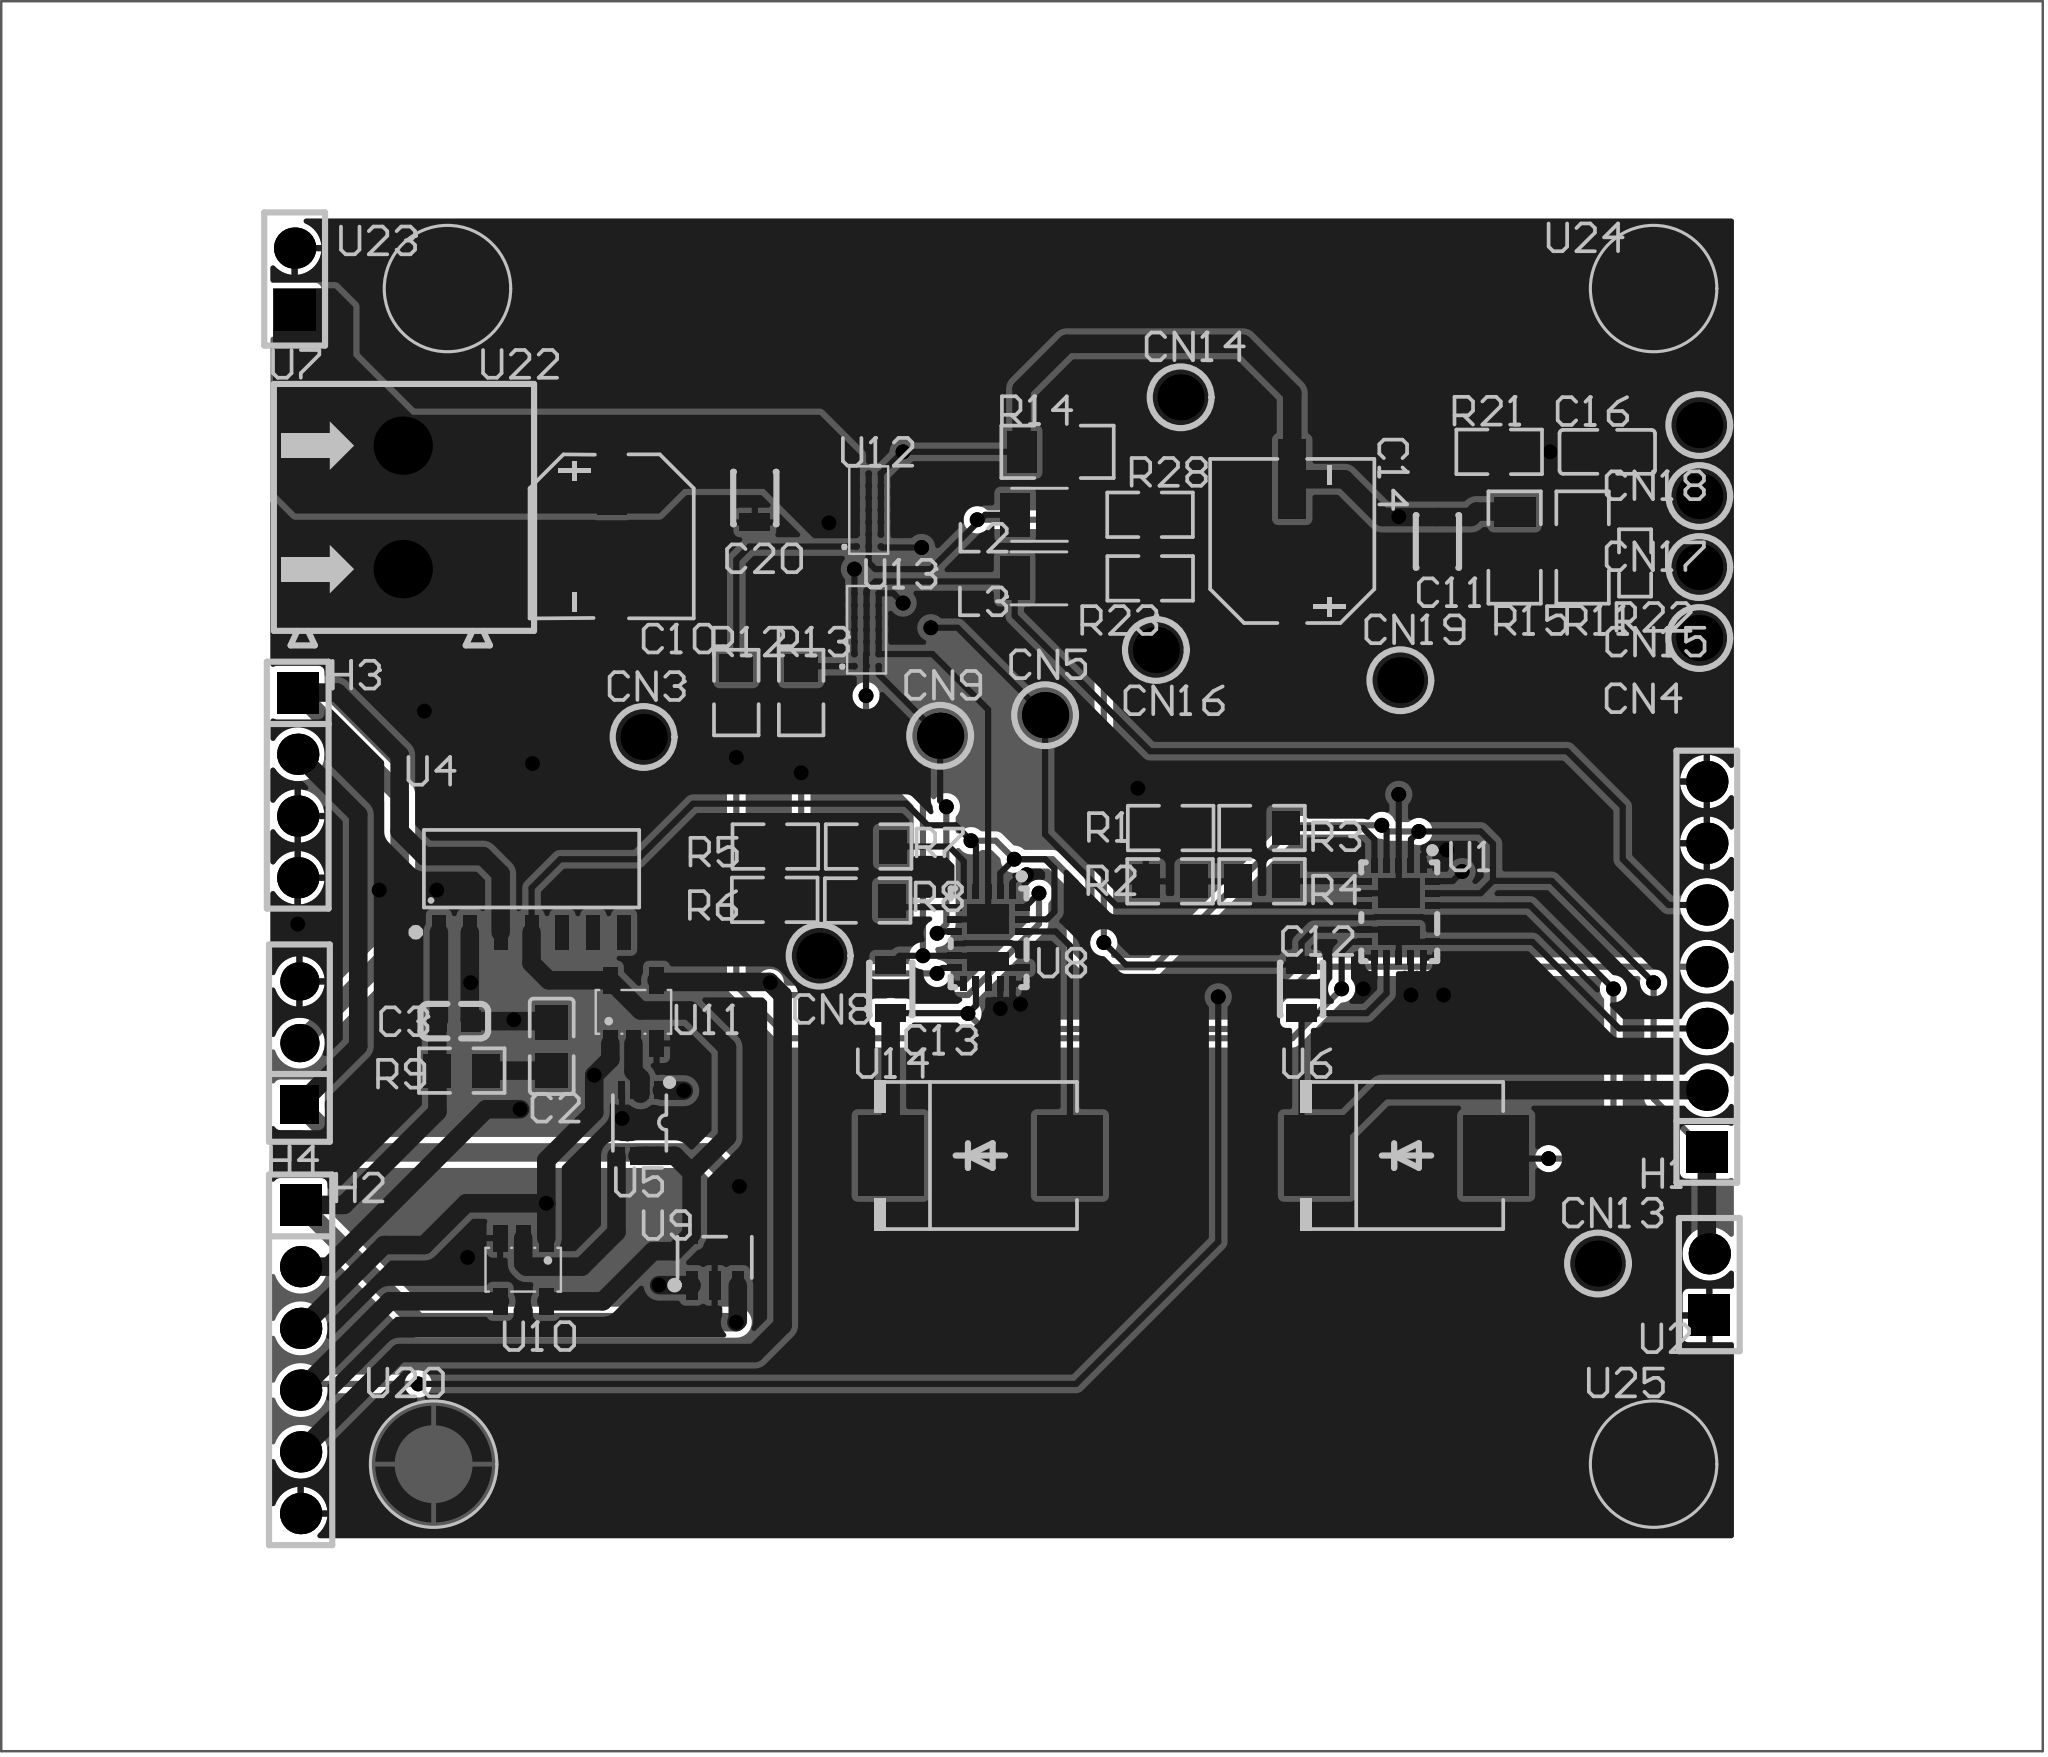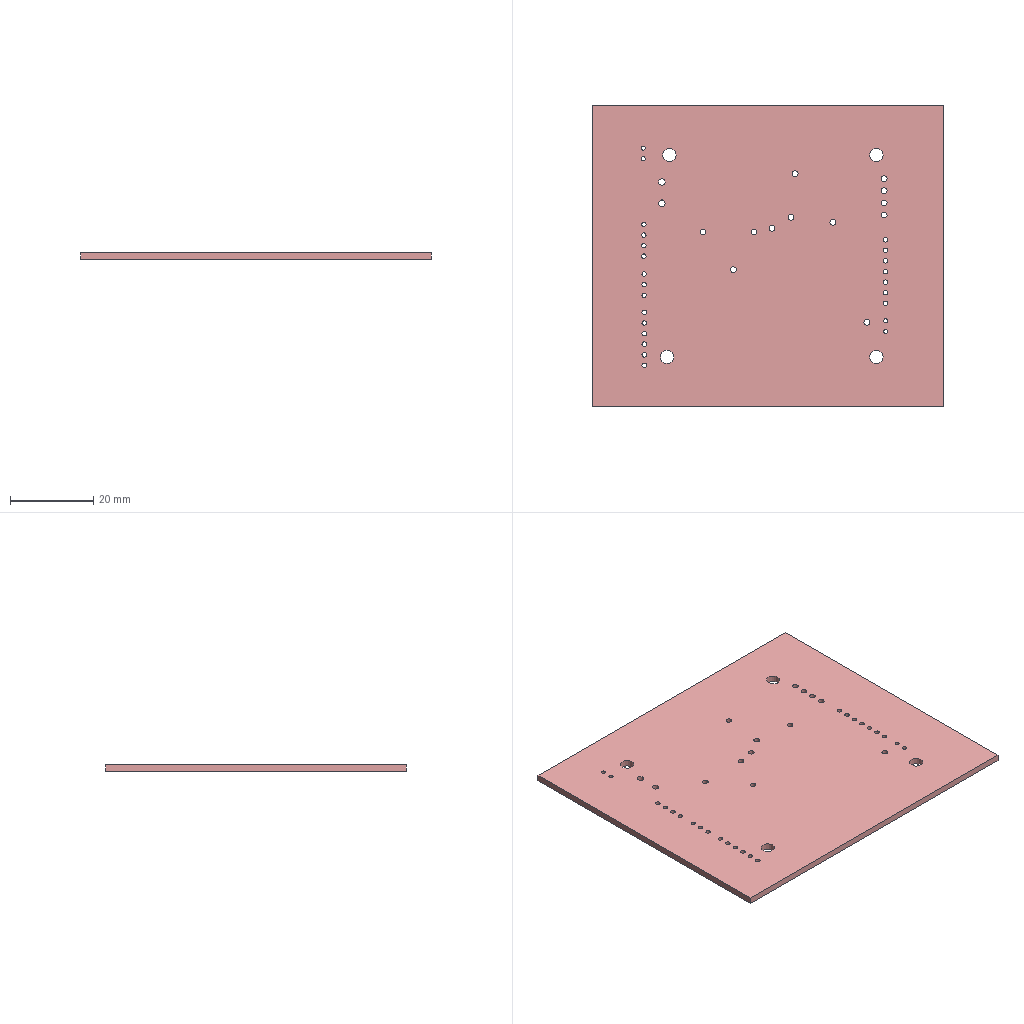Circuit board layout | Altium Designer | box 83.9 x 72 x 1.6 mm
Layer stack:
# Altium Designer layer stack of  (unit mm; dielectric type: 0 none, 1 core, 2 prepreg, 3 surface material)
index,name,kind,layer,copper_thickness_mm,dielectric_type,dielectric_thickness_mm,dielectric_material,dielectric_constant
0,Top Paste Mask Layer,other,,,,,,
1,Top Silkscreen Layer,other,,,,,,
2,Top Solder Mask Layer,dielectric,,,3,0.01,,3.3
3,Top Layer,copper,Top Layer,0.035,,,,
4,Dielectric1,dielectric,,,3,1.51,FR4,4.5
5,Bottom Layer,copper,Bottom Layer,0.035,,,,
6,Bottom Solder Mask Layer,dielectric,,,3,0.01,,3.3
7,Bottom Silkscreen Layer,other,,,,,,
8,Bottom Paste Mask Layer,other,,,,,,
# drill layer pairs: low layer,high layer
drill_pair,Top Layer,Bottom Layer
Part placement:
Designator,Comment,Layer,Footprint,Center-X(mm),Center-Y(mm),Rotation
C2,24pF,TopLayer,C0805,92.485,98.854,90
C3,0.6pF,TopLayer,C0603,88.48,99.891,0
C10,100uF,TopLayer,CAP-SMD_BD6.3-L6.6-W6.6-LS7.3-FD-H7.7,94.95,119.837,270
C11,100nF,TopLayer,CAP-SMD_L2.0-W1.25,128.905,119.634,270
C12,100nF,TopLayer,CAP-SMD_L2.0-W1.25,123.317,101.219,270
C13,100nF,TopLayer,CAP-SMD_L2.0-W1.25,106.426,101.219,270
C14,100uF,TopLayer,CAP-SMD_BD6.3-L6.6-W6.6-RD,122.936,119.634,270
C16,1.2pF,TopLayer,C0805,135.89,123.317,0
C20,100nF,TopLayer,CAP-SMD_L2.0-W1.25,100.838,121.412,90
H1,PZ254V-11-07P,TopLayer,HDR-TH_7P-P2.54-V-M,139.984,102.13,90
H2,PZ254V-11-06P,TopLayer,HDR-TH_6P-P2.54-V-M,82.161,85.979,270
H3,PZ254V-11-04P,TopLayer,HDR-TH_4P-P2.54-V-M,82.042,109.601,270
H4,PM254V-11-03-H85,TopLayer,HDR-TH_3P-P2.54-V-F,82.111,98.987,90
L2,100nH,TopLayer,IND-SMD_L2.3-W1.8,112.541,120.727,0
L3,100nH,TopLayer,IND-SMD_L2.3-W1.8,112.522,118.11,0
R1,120kΩ,TopLayer,R0805,117.936,107.838,0
R2,120kΩ,TopLayer,R0805,117.911,105.644,0
R3,20kΩ,TopLayer,R0805,121.693,107.838,0
R4,20kΩ,TopLayer,R0805,121.693,105.644,0
R5,120kΩ,TopLayer,R0805,101.68,107.076,0
R6,120kΩ,TopLayer,R0805,101.655,104.882,0
R7,20kΩ,TopLayer,R0805,105.516,107.076,0
R8,20kΩ,TopLayer,R0805,105.478,104.854,0
R9,100kΩ,TopLayer,R0805,88.786,97.854,0
R11,900kΩ,TopLayer,R1206,134.874,119.38,270
R12,4.7Ω,TopLayer,R0805,100.076,113.411,90
R13,4.7Ω,TopLayer,R0805,102.743,113.411,90
R14,0Ω,TopLayer,R1206,113.284,123.317,180
R15,600mΩ,TopLayer,R1206,132.08,119.38,270
R21,1.8MΩ,TopLayer,R0805,131.445,123.317,0
R22,69kΩ,TopLayer,R0603,137.033,118.745,270
R23,10mΩ,TopLayer,R0805,117.094,118.11,0
R28,10mΩ,TopLayer,R0805,117.088,120.727,0
U1,LMG1210RVRR,TopLayer,WQFN-19_L4.0-W3.0-P0.50-BL-EP_LMG1210RVRR,127.316,104.403,270
U2,ZX-PM2.54-1-2PY,TopLayer,HDR-TH_2P-P2.54-V-F,140.085,89.049,90
U4,AD8574ARZ-REEL7-HXY,TopLayer,SOP-14_L8.7-W3.9-P1.27-LS6.0-BL,91.657,106.163,0
U5,SN74LVC1G74DCUR,TopLayer,SSOP-8_L2.0-W2.3-P0.50-LS3.1-BR,96.1,95.7,90
U6,B540C,TopLayer,SMC_L6.9-W5.9-LS7.9-RD,127.635,94.361,0
U7,ZX-PM2.54-1-2PY,TopLayer,HDR-TH_2P-P2.54-V-F,81.915,130.429,90
U8,LMG1210RVRR,TopLayer,WQFN-19_L4.0-W3.0-P0.50-BL-EP_LMG1210RVRR,110.43,103.33,270
U9,LTC6752HS5#TRMPBF,TopLayer,SOT-23-5_L3.0-W1.7-P0.95-LS2.8-BL,99.187,90.17,0
U10,SN74LVC1G08DBVR,TopLayer,SOT-23-5_L3.0-W1.7-P0.95-LS2.8-BR,91.313,89.662,90
U11,SN74LVC1G08DBVR,TopLayer,SOT-23-5_L3.0-W1.7-P0.95-LS2.8-BR,95.846,100.272,270
U12,,TopLayer,2111,105.521,120.92,90
U13,,TopLayer,2111,105.433,115.997,90
U14,B540C,TopLayer,SMC_L6.9-W5.9-LS7.9-RD,110.109,94.361,0
U20,M3x10+6Cu,TopLayer,SMD_L4.7-W4.7-D3.0,87.63,81.661,0
U22,KF128-5.08-2P-AA,TopLayer,CONN-TH_P5.08_KF128-5.08-2P,86.36,121.031,270
U23,M3x10+6Cu,TopLayer,SMD_L4.7-W4.7-D3.0,88.2,130.036,0
U24,M3x10+6Cu,TopLayer,SMD_L4.7-W4.7-D3.0,137.795,130.036,0
U25,M3x10+6Cu,TopLayer,SMD_L4.7-W4.7-D3.0,137.795,81.661,0
CN3,RH-5001,TopLayer,TEST-TH_BD2.54-P1.4_BLACK,96.263,111.584,0
CN4,RH-5001,TopLayer,TEST-TH_BD2.54-P1.4_BLACK,139.673,115.656,0
CN5,RH-5001,TopLayer,TEST-TH_BD2.54-P1.4_BLACK,112.773,112.481,0
CN8,RH-5001,TopLayer,TEST-TH_BD2.54-P1.4_BLACK,103.502,102.582,0
CN9,RH-5001,TopLayer,TEST-TH_BD2.54-P1.4_BLACK,108.458,111.633,0
CN13,RH-5001,TopLayer,TEST-TH_BD2.54-P1.4_BLACK,135.509,89.916,0
CN14,RH-5001,TopLayer,TEST-TH_BD2.54-P1.4_BLACK,118.346,125.561,0
CN15,RH-5001,TopLayer,TEST-TH_BD2.54-P1.4_BLACK,139.673,118.576,0
CN16,RH-5001,TopLayer,TEST-TH_BD2.54-P1.4_BLACK,117.329,115.163,0
CN17,RH-5001,TopLayer,TEST-TH_BD2.54-P1.4_BLACK,139.673,121.498,0
CN18,RH-5001,TopLayer,TEST-TH_BD2.54-P1.4_BLACK,139.673,124.418,0
CN19,RH-5001,TopLayer,TEST-TH_BD2.54-P1.4_BLACK,127.381,113.919,0
Pad and via stacks:
# Altium Designer via and pad stacks of  (unit mm). Each distinct definition once, with the count of objects using it.
# via: kind,start_layer,end_layer,hole_mm,diameter_mm,mode(0 simple;1 top-mid-bottom;2 full stack),diameter_per_layer,count,example_net
# pad: kind,layer,hole_mm,hole_type(0 round;1 square;2 slot),plating,top_size,top_shape(1 round;2 rect;3 octagon;9 rounded rect),mid_size,bottom_size,mode,footprint,size_per_layer,count,example
pad,Top Layer,0,0,plated,1.41x1.35,2,1.41x1.35,1.41x1.35,0,C0805,,4,C2.2
pad,Top Layer,0,0,plated,0.8x0.9,2,0.8x0.9,0.8x0.9,0,C0603,,2,C3.2
pad,Top Layer,0,0,plated,3.5x1.2,2,3.5x1.2,3.5x1.2,0,CAP-SMD_BD6.3-L6.6-W6.6-LS7.3-FD-H7.7,,2,C10.1
pad,Top Layer,0,0,plated,1.25x0.7,2,1.25x0.7,1.25x0.7,0,CAP-SMD_L2.0-W1.25,,8,C11.1
pad,Top Layer,0,0,plated,3.26x1.15,2,3.26x1.15,3.26x1.15,0,CAP-SMD_BD6.3-L6.6-W6.6-RD,,2,C14.2
pad,Top Layer,0,0,plated,1.8x1.2,2,1.8x1.2,1.8x1.2,0,IND-SMD_L2.3-W1.8,,4,L2.1
pad,Top Layer,0,0,plated,1.133x1.377,2,1.133x1.377,1.133x1.377,0,R0805,,28,R1.2
pad,Top Layer,0,0,plated,1.208x1.701,2,1.208x1.701,1.208x1.701,0,R1206,,6,R11.2
pad,Top Layer,0,0,plated,0.8065x0.864,2,0.8065x0.864,0.8065x0.864,0,R0603,,2,R22.2
pad,Top Layer,0,0,plated,0.6x0.25,2,0.6x0.25,0.6x0.25,0,WQFN-19_L4.0-W3.0-P0.50-BL-EP_LMG1210RVRR,,38,U1.1
pad,Top Layer,0,0,plated,1.7x1.2,2,1.7x1.2,1.7x1.2,0,WQFN-19_L4.0-W3.0-P0.50-BL-EP_LMG1210RVRR,,2,U1.20
pad,Top Layer,0,0,plated,1.7x0.75,2,1.7x0.75,1.7x0.75,0,WQFN-19_L4.0-W3.0-P0.50-BL-EP_LMG1210RVRR,,2,U1.21
pad,Top Layer,0,0,plated,0.56x1.43,2,0.56x1.43,0.56x1.43,0,SOP-14_L8.7-W3.9-P1.27-LS6.0-BL,,14,U4.1
pad,Top Layer,0,0,plated,0.7x0.26,2,0.7x0.26,0.7x0.26,0,SSOP-8_L2.0-W2.3-P0.50-LS3.1-BR,,8,U5.1
pad,Top Layer,0,0,plated,2.7x3.3,2,2.7x3.3,2.7x3.3,0,SMC_L6.9-W5.9-LS7.9-RD,,4,U6.2
pad,Top Layer,0,0,plated,0.49x1.157,2,0.49x1.157,0.49x1.157,0,SOT-23-5_L3.0-W1.7-P0.95-LS2.8-BL,,3,U9.1
pad,Top Layer,0,0,plated,0.49x1.175,2,0.49x1.175,0.49x1.175,0,SOT-23-5_L3.0-W1.7-P0.95-LS2.8-BL,,2,U9.4
pad,Top Layer,0,0,plated,1.1x0.6,2,1.1x0.6,1.1x0.6,0,SOT-23-5_L3.0-W1.7-P0.95-LS2.8-BR,,10,U10.5
pad,Top Layer,0,0,plated,0.1369x0.1369,1,0.1369x0.1369,0.1369x0.1369,0,2111,,40,U12.5
pad,Top Layer,0,0,plated,0.2753x0.276,3,0.2753x0.276,0.2753x0.276,0,2111,,2,U12.4
pad,Top Layer,0,0,plated,0.2488x0.2488,1,0.2488x0.2488,0.2488x0.2488,0,SMD_L4.7-W4.7-D3.0,,16,U20.1
pad,Multi-Layer,1.1,0,plated,1.7x1.7,2,1.7x1.7,1.7x1.7,0,HDR-TH_7P-P2.54-V-M,,1,H1.1
pad,Multi-Layer,1.1,0,plated,1.7x1.7,1,1.7x1.7,1.7x1.7,0,HDR-TH_7P-P2.54-V-M,,6,H1.2
pad,Multi-Layer,1.1,0,plated,1.7x1.7,2,1.7x1.7,1.7x1.7,0,HDR-TH_6P-P2.54-V-M,,1,H2.1
pad,Multi-Layer,1.1,0,plated,1.7x1.7,1,1.7x1.7,1.7x1.7,0,HDR-TH_6P-P2.54-V-M,,5,H2.2
pad,Multi-Layer,1.1,0,plated,1.7x1.7,2,1.7x1.7,1.7x1.7,0,HDR-TH_4P-P2.54-V-M,,1,H3.1
pad,Multi-Layer,1.1,0,plated,1.7x1.7,1,1.7x1.7,1.7x1.7,0,HDR-TH_4P-P2.54-V-M,,3,H3.2
pad,Multi-Layer,1.02,0,plated,1.575x1.575,1,1.575x1.575,1.575x1.575,0,HDR-TH_3P-P2.54-V-F,,2,H4.3
pad,Multi-Layer,1.02,0,plated,1.575x1.575,2,1.575x1.575,1.575x1.575,0,HDR-TH_3P-P2.54-V-F,,1,H4.1
pad,Multi-Layer,1,0,plated,1.7x1.7,2,1.7x1.7,1.7x1.7,0,HDR-TH_2P-P2.54-V-F,,2,U2.1
pad,Multi-Layer,1,0,plated,1.7x1.7,1,1.7x1.7,1.7x1.7,0,HDR-TH_2P-P2.54-V-F,,2,U2.2
pad,Multi-Layer,1.6,0,plated,2.4x2.4,1,2.4x2.4,2.4x2.4,0,CONN-TH_P5.08_KF128-5.08-2P,,2,U22.1
pad,Multi-Layer,1.39,0,plated,1.9x1.9,1,1.9x1.9,1.9x1.9,0,TEST-TH_BD2.54-P1.4_BLACK,,12,CN3.1
via,Top Layer,Bottom Layer,0.3048,0.61,0,,56,VIN
Copper pours:
name,layer,net,type(0 solid;1 hatched;2 none)
Top Layer-GND,Top Layer,GND,0
Bottom Layer-GND,Bottom Layer,GND,0